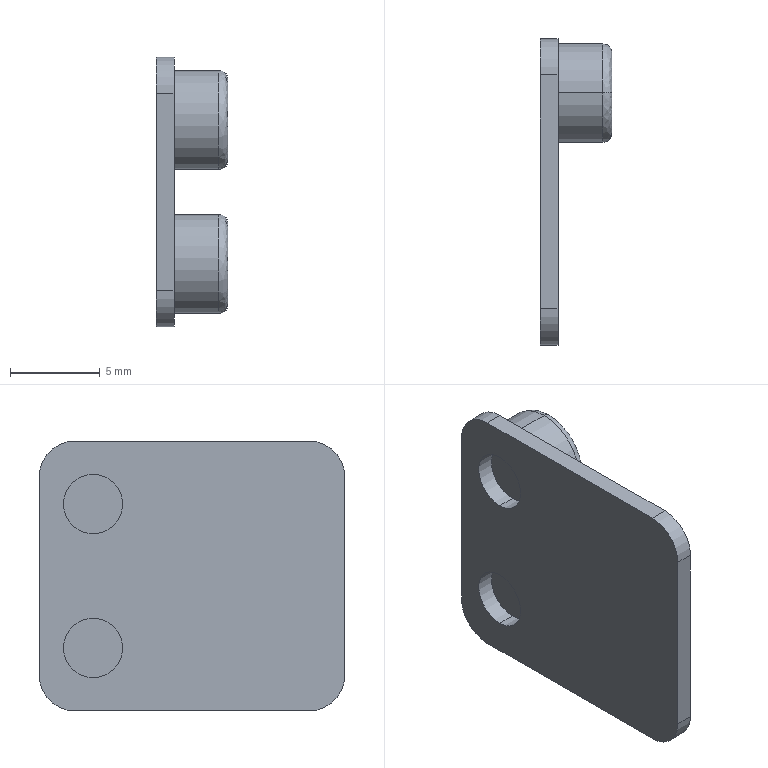Part | SolidWorks | features BaseBody 1 | 1 solid | 40 faces | box 4 x 17 x 15 mm | volume 361.162 mm3 | plane 24 | cylinder 12 | spline 4 | commonest cylinder face diameters 3.3 x4 4 x4 5.5 x4
STEP:
#1=CARTESIAN_POINT('',(4.,5.,1.25));
#2=VERTEX_POINT('',#1);
#3=CARTESIAN_POINT('',(4.,5.,5.75));
#4=VERTEX_POINT('',#3);
#5=CARTESIAN_POINT('',(4.,5.,1.25));
#6=CARTESIAN_POINT('',(4.,0.5,1.25));
#7=CARTESIAN_POINT('',(4.,0.5,5.75));
#8=CARTESIAN_POINT('',(4.,5.,5.75));
#9=(BOUNDED_CURVE()B_SPLINE_CURVE(3,(#5,#6,#7,#8),.UNSPECIFIED.,.F.,.T.)B_SPLINE_CURVE_WITH_KNOTS((4,4),(0.,0.5),.UNSPECIFIED.)CURVE()GEOMETRIC_REPRESENTATION_ITEM()RATIONAL_B_SPLINE_CURVE((1.,0.3333,0.3333,1.))REPRESENTATION_ITEM(''));
#10=EDGE_CURVE('',#2,#4,#9,.T.);
#11=ORIENTED_EDGE('',*,*,#10,.T.);
#12=CARTESIAN_POINT('',(3.5,5.,6.25));
#13=VERTEX_POINT('',#12);
#14=CARTESIAN_POINT('',(3.5,5.,5.75));
#15=DIRECTION('',(0.,-1.,0.));
#16=DIRECTION('',(0.,0.,1.));
#17=AXIS2_PLACEMENT_3D('',#14,#15,#16);
#18=CIRCLE('',#17,0.5);
#19=EDGE_CURVE('',#4,#13,#18,.T.);
#20=ORIENTED_EDGE('',*,*,#19,.T.);
#21=CARTESIAN_POINT('',(3.5,5.,0.75));
#22=VERTEX_POINT('',#21);
#23=CARTESIAN_POINT('',(3.5,5.,3.5));
#24=DIRECTION('',(-1.,0.,0.));
#25=DIRECTION('',(0.,0.,1.));
#26=AXIS2_PLACEMENT_3D('',#23,#24,#25);
#27=CIRCLE('',#26,2.75);
#28=EDGE_CURVE('',#22,#13,#27,.T.);
#29=ORIENTED_EDGE('',*,*,#28,.F.);
#30=CARTESIAN_POINT('',(3.5,5.,1.25));
#31=DIRECTION('',(0.,1.,0.));
#32=DIRECTION('',(0.,0.,-1.));
#33=AXIS2_PLACEMENT_3D('',#30,#31,#32);
#34=CIRCLE('',#33,0.5);
#35=EDGE_CURVE('',#2,#22,#34,.T.);
#36=ORIENTED_EDGE('',*,*,#35,.F.);
#37=EDGE_LOOP('',(#11,#20,#29,#36));
#38=FACE_OUTER_BOUND('',#37,.T.);
#39=CARTESIAN_POINT('',(4.,5.,5.75));
#40=CARTESIAN_POINT('',(4.,0.5,5.75));
#41=CARTESIAN_POINT('',(4.,0.5,1.25));
#42=CARTESIAN_POINT('',(4.,5.,1.25));
#43=CARTESIAN_POINT('',(4.,5.,6.043));
#44=CARTESIAN_POINT('',(4.,-0.08579,6.043));
#45=CARTESIAN_POINT('',(4.,-0.08579,0.9571));
#46=CARTESIAN_POINT('',(4.,5.,0.9571));
#47=CARTESIAN_POINT('',(3.793,5.,6.25));
#48=CARTESIAN_POINT('',(3.793,-0.5,6.25));
#49=CARTESIAN_POINT('',(3.793,-0.5,0.75));
#50=CARTESIAN_POINT('',(3.793,5.,0.75));
#51=CARTESIAN_POINT('',(3.5,5.,6.25));
#52=CARTESIAN_POINT('',(3.5,-0.5,6.25));
#53=CARTESIAN_POINT('',(3.5,-0.5,0.75));
#54=CARTESIAN_POINT('',(3.5,5.,0.75));
#55=(BOUNDED_SURFACE()B_SPLINE_SURFACE(3,3,((#39,#40,#41,#42),(#43,#44,#45,#46),(#47,#48,#49,#50),(#51,#52,#53,#54)),.UNSPECIFIED.,.F.,.F.,.F.)B_SPLINE_SURFACE_WITH_KNOTS((4,4),(4,4),(0.,1.),(0.,1.),.UNSPECIFIED.)GEOMETRIC_REPRESENTATION_ITEM()RATIONAL_B_SPLINE_SURFACE(((1.,0.3333,0.3333,1.),(0.8047,0.2682,0.2682,0.8047),(0.8047,0.2682,0.2682,0.8047),(1.,0.3333,0.3333,1.)))REPRESENTATION_ITEM('')SURFACE());
#56=ADVANCED_FACE('',(#38),#55,.T.);
#57=CARTESIAN_POINT('',(4.,5.,9.25));
#58=VERTEX_POINT('',#57);
#59=CARTESIAN_POINT('',(4.,5.,13.75));
#60=VERTEX_POINT('',#59);
#61=CARTESIAN_POINT('',(4.,5.,9.25));
#62=CARTESIAN_POINT('',(4.,0.5,9.25));
#63=CARTESIAN_POINT('',(4.,0.5,13.75));
#64=CARTESIAN_POINT('',(4.,5.,13.75));
#65=(BOUNDED_CURVE()B_SPLINE_CURVE(3,(#61,#62,#63,#64),.UNSPECIFIED.,.F.,.F.)B_SPLINE_CURVE_WITH_KNOTS((4,4),(0.,0.5),.UNSPECIFIED.)CURVE()GEOMETRIC_REPRESENTATION_ITEM()RATIONAL_B_SPLINE_CURVE((1.,0.3333,0.3333,1.))REPRESENTATION_ITEM(''));
#66=EDGE_CURVE('',#58,#60,#65,.T.);
#67=ORIENTED_EDGE('',*,*,#66,.T.);
#68=CARTESIAN_POINT('',(3.5,5.,14.25));
#69=VERTEX_POINT('',#68);
#70=CARTESIAN_POINT('',(3.5,5.,13.75));
#71=DIRECTION('',(0.,-1.,0.));
#72=DIRECTION('',(0.,0.,1.));
#73=AXIS2_PLACEMENT_3D('',#70,#71,#72);
#74=CIRCLE('',#73,0.5);
#75=EDGE_CURVE('',#60,#69,#74,.T.);
#76=ORIENTED_EDGE('',*,*,#75,.T.);
#77=CARTESIAN_POINT('',(3.5,5.,8.75));
#78=VERTEX_POINT('',#77);
#79=CARTESIAN_POINT('',(3.5,5.,11.5));
#80=DIRECTION('',(-1.,0.,0.));
#81=DIRECTION('',(0.,0.,1.));
#82=AXIS2_PLACEMENT_3D('',#79,#80,#81);
#83=CIRCLE('',#82,2.75);
#84=EDGE_CURVE('',#78,#69,#83,.T.);
#85=ORIENTED_EDGE('',*,*,#84,.F.);
#86=CARTESIAN_POINT('',(3.5,5.,9.25));
#87=DIRECTION('',(0.,1.,0.));
#88=DIRECTION('',(0.,0.,-1.));
#89=AXIS2_PLACEMENT_3D('',#86,#87,#88);
#90=CIRCLE('',#89,0.5);
#91=EDGE_CURVE('',#58,#78,#90,.T.);
#92=ORIENTED_EDGE('',*,*,#91,.F.);
#93=EDGE_LOOP('',(#67,#76,#85,#92));
#94=FACE_OUTER_BOUND('',#93,.T.);
#95=CARTESIAN_POINT('',(4.,5.,13.75));
#96=CARTESIAN_POINT('',(4.,0.5,13.75));
#97=CARTESIAN_POINT('',(4.,0.5,9.25));
#98=CARTESIAN_POINT('',(4.,5.,9.25));
#99=CARTESIAN_POINT('',(4.,5.,14.043));
#100=CARTESIAN_POINT('',(4.,-0.08579,14.043));
#101=CARTESIAN_POINT('',(4.,-0.08579,8.957));
#102=CARTESIAN_POINT('',(4.,5.,8.957));
#103=CARTESIAN_POINT('',(3.793,5.,14.25));
#104=CARTESIAN_POINT('',(3.793,-0.5,14.25));
#105=CARTESIAN_POINT('',(3.793,-0.5,8.75));
#106=CARTESIAN_POINT('',(3.793,5.,8.75));
#107=CARTESIAN_POINT('',(3.5,5.,14.25));
#108=CARTESIAN_POINT('',(3.5,-0.5,14.25));
#109=CARTESIAN_POINT('',(3.5,-0.5,8.75));
#110=CARTESIAN_POINT('',(3.5,5.,8.75));
#111=(BOUNDED_SURFACE()B_SPLINE_SURFACE(3,3,((#95,#96,#97,#98),(#99,#100,#101,#102),(#103,#104,#105,#106),(#107,#108,#109,#110)),.UNSPECIFIED.,.F.,.F.,.T.)B_SPLINE_SURFACE_WITH_KNOTS((4,4),(4,4),(0.,1.),(0.,1.),.UNSPECIFIED.)GEOMETRIC_REPRESENTATION_ITEM()RATIONAL_B_SPLINE_SURFACE(((1.,0.3333,0.3333,1.),(0.8047,0.2682,0.2682,0.8047),(0.8047,0.2682,0.2682,0.8047),(1.,0.3333,0.3333,1.)))REPRESENTATION_ITEM('')SURFACE());
#112=ADVANCED_FACE('',(#94),#111,.T.);
#113=CARTESIAN_POINT('',(0.,5.,1.85));
#114=VERTEX_POINT('',#113);
#115=CARTESIAN_POINT('',(0.,5.,5.15));
#116=VERTEX_POINT('',#115);
#117=CARTESIAN_POINT('',(0.,5.,3.5));
#118=DIRECTION('',(-1.,0.,0.));
#119=DIRECTION('',(0.,0.,-1.));
#120=AXIS2_PLACEMENT_3D('',#117,#118,#119);
#121=CIRCLE('',#120,1.65);
#122=EDGE_CURVE('',#114,#116,#121,.T.);
#123=ORIENTED_EDGE('',*,*,#122,.T.);
#124=CARTESIAN_POINT('',(1.,5.,5.15));
#125=VERTEX_POINT('',#124);
#126=CARTESIAN_POINT('',(0.,5.,5.15));
#127=DIRECTION('',(1.,0.,0.));
#128=VECTOR('',#127,1000.);
#129=LINE('',#126,#128);
#130=EDGE_CURVE('',#116,#125,#129,.T.);
#131=ORIENTED_EDGE('',*,*,#130,.T.);
#132=CARTESIAN_POINT('',(1.,5.,1.85));
#133=VERTEX_POINT('',#132);
#134=CARTESIAN_POINT('',(1.,5.,3.5));
#135=DIRECTION('',(-1.,0.,0.));
#136=DIRECTION('',(0.,0.,-1.));
#137=AXIS2_PLACEMENT_3D('',#134,#135,#136);
#138=CIRCLE('',#137,1.65);
#139=EDGE_CURVE('',#133,#125,#138,.T.);
#140=ORIENTED_EDGE('',*,*,#139,.F.);
#141=CARTESIAN_POINT('',(0.,5.,1.85));
#142=DIRECTION('',(1.,0.,0.));
#143=VECTOR('',#142,1000.);
#144=LINE('',#141,#143);
#145=EDGE_CURVE('',#114,#133,#144,.T.);
#146=ORIENTED_EDGE('',*,*,#145,.F.);
#147=EDGE_LOOP('',(#123,#131,#140,#146));
#148=FACE_OUTER_BOUND('',#147,.T.);
#149=CARTESIAN_POINT('',(0.,5.,3.5));
#150=DIRECTION('',(1.,0.,0.));
#151=DIRECTION('',(0.,0.,-1.));
#152=AXIS2_PLACEMENT_3D('',#149,#150,#151);
#153=CYLINDRICAL_SURFACE('',#152,1.65);
#154=ADVANCED_FACE('',(#148),#153,.F.);
#155=CARTESIAN_POINT('',(0.,5.,9.85));
#156=VERTEX_POINT('',#155);
#157=CARTESIAN_POINT('',(0.,5.,13.15));
#158=VERTEX_POINT('',#157);
#159=CARTESIAN_POINT('',(0.,5.,11.5));
#160=DIRECTION('',(-1.,0.,0.));
#161=DIRECTION('',(0.,0.,-1.));
#162=AXIS2_PLACEMENT_3D('',#159,#160,#161);
#163=CIRCLE('',#162,1.65);
#164=EDGE_CURVE('',#156,#158,#163,.T.);
#165=ORIENTED_EDGE('',*,*,#164,.T.);
#166=CARTESIAN_POINT('',(1.,5.,13.15));
#167=VERTEX_POINT('',#166);
#168=CARTESIAN_POINT('',(0.,5.,13.15));
#169=DIRECTION('',(1.,0.,0.));
#170=VECTOR('',#169,1000.);
#171=LINE('',#168,#170);
#172=EDGE_CURVE('',#158,#167,#171,.T.);
#173=ORIENTED_EDGE('',*,*,#172,.T.);
#174=CARTESIAN_POINT('',(1.,5.,9.85));
#175=VERTEX_POINT('',#174);
#176=CARTESIAN_POINT('',(1.,5.,11.5));
#177=DIRECTION('',(-1.,0.,0.));
#178=DIRECTION('',(0.,0.,-1.));
#179=AXIS2_PLACEMENT_3D('',#176,#177,#178);
#180=CIRCLE('',#179,1.65);
#181=EDGE_CURVE('',#175,#167,#180,.T.);
#182=ORIENTED_EDGE('',*,*,#181,.F.);
#183=CARTESIAN_POINT('',(0.,5.,9.85));
#184=DIRECTION('',(1.,0.,0.));
#185=VECTOR('',#184,1000.);
#186=LINE('',#183,#185);
#187=EDGE_CURVE('',#156,#175,#186,.T.);
#188=ORIENTED_EDGE('',*,*,#187,.F.);
#189=EDGE_LOOP('',(#165,#173,#182,#188));
#190=FACE_OUTER_BOUND('',#189,.T.);
#191=CARTESIAN_POINT('',(0.,5.,11.5));
#192=DIRECTION('',(1.,0.,0.));
#193=DIRECTION('',(0.,0.,-1.));
#194=AXIS2_PLACEMENT_3D('',#191,#192,#193);
#195=CYLINDRICAL_SURFACE('',#194,1.65);
#196=ADVANCED_FACE('',(#190),#195,.F.);
#197=CARTESIAN_POINT('',(3.5,5.,3.5));
#198=DIRECTION('',(-1.,0.,0.));
#199=DIRECTION('',(0.,0.,1.));
#200=AXIS2_PLACEMENT_3D('',#197,#198,#199);
#201=CIRCLE('',#200,2.75);
#202=EDGE_CURVE('',#13,#22,#201,.T.);
#203=ORIENTED_EDGE('',*,*,#202,.T.);
#204=CARTESIAN_POINT('',(1.,5.,0.75));
#205=VERTEX_POINT('',#204);
#206=CARTESIAN_POINT('',(4.,5.,0.75));
#207=DIRECTION('',(-1.,0.,0.));
#208=VECTOR('',#207,1000.);
#209=LINE('',#206,#208);
#210=EDGE_CURVE('',#22,#205,#209,.T.);
#211=ORIENTED_EDGE('',*,*,#210,.T.);
#212=CARTESIAN_POINT('',(1.,5.,6.25));
#213=VERTEX_POINT('',#212);
#214=CARTESIAN_POINT('',(1.,5.,3.5));
#215=DIRECTION('',(-1.,0.,0.));
#216=DIRECTION('',(0.,0.,1.));
#217=AXIS2_PLACEMENT_3D('',#214,#215,#216);
#218=CIRCLE('',#217,2.75);
#219=EDGE_CURVE('',#213,#205,#218,.T.);
#220=ORIENTED_EDGE('',*,*,#219,.F.);
#221=CARTESIAN_POINT('',(4.,5.,6.25));
#222=DIRECTION('',(-1.,0.,0.));
#223=VECTOR('',#222,1000.);
#224=LINE('',#221,#223);
#225=EDGE_CURVE('',#13,#213,#224,.T.);
#226=ORIENTED_EDGE('',*,*,#225,.F.);
#227=EDGE_LOOP('',(#203,#211,#220,#226));
#228=FACE_OUTER_BOUND('',#227,.T.);
#229=CARTESIAN_POINT('',(4.,5.,3.5));
#230=DIRECTION('',(-1.,0.,0.));
#231=DIRECTION('',(0.,0.,1.));
#232=AXIS2_PLACEMENT_3D('',#229,#230,#231);
#233=CYLINDRICAL_SURFACE('',#232,2.75);
#234=ADVANCED_FACE('',(#228),#233,.T.);
#235=CARTESIAN_POINT('',(3.5,5.,11.5));
#236=DIRECTION('',(-1.,0.,0.));
#237=DIRECTION('',(0.,0.,1.));
#238=AXIS2_PLACEMENT_3D('',#235,#236,#237);
#239=CIRCLE('',#238,2.75);
#240=EDGE_CURVE('',#69,#78,#239,.T.);
#241=ORIENTED_EDGE('',*,*,#240,.T.);
#242=CARTESIAN_POINT('',(1.,5.,8.75));
#243=VERTEX_POINT('',#242);
#244=CARTESIAN_POINT('',(4.,5.,8.75));
#245=DIRECTION('',(-1.,0.,0.));
#246=VECTOR('',#245,1000.);
#247=LINE('',#244,#246);
#248=EDGE_CURVE('',#78,#243,#247,.T.);
#249=ORIENTED_EDGE('',*,*,#248,.T.);
#250=CARTESIAN_POINT('',(1.,5.,14.25));
#251=VERTEX_POINT('',#250);
#252=CARTESIAN_POINT('',(1.,5.,11.5));
#253=DIRECTION('',(-1.,0.,0.));
#254=DIRECTION('',(0.,0.,1.));
#255=AXIS2_PLACEMENT_3D('',#252,#253,#254);
#256=CIRCLE('',#255,2.75);
#257=EDGE_CURVE('',#251,#243,#256,.T.);
#258=ORIENTED_EDGE('',*,*,#257,.F.);
#259=CARTESIAN_POINT('',(4.,5.,14.25));
#260=DIRECTION('',(-1.,0.,0.));
#261=VECTOR('',#260,1000.);
#262=LINE('',#259,#261);
#263=EDGE_CURVE('',#69,#251,#262,.T.);
#264=ORIENTED_EDGE('',*,*,#263,.F.);
#265=EDGE_LOOP('',(#241,#249,#258,#264));
#266=FACE_OUTER_BOUND('',#265,.T.);
#267=CARTESIAN_POINT('',(4.,5.,11.5));
#268=DIRECTION('',(-1.,0.,0.));
#269=DIRECTION('',(0.,0.,1.));
#270=AXIS2_PLACEMENT_3D('',#267,#268,#269);
#271=CYLINDRICAL_SURFACE('',#270,2.75);
#272=ADVANCED_FACE('',(#266),#271,.T.);
#273=CARTESIAN_POINT('',(0.,-7.,15.));
#274=VERTEX_POINT('',#273);
#275=CARTESIAN_POINT('',(0.,-9.,13.));
#276=VERTEX_POINT('',#275);
#277=CARTESIAN_POINT('',(0.,-7.,13.));
#278=DIRECTION('',(1.,0.,0.));
#279=DIRECTION('',(0.,0.,1.));
#280=AXIS2_PLACEMENT_3D('',#277,#278,#279);
#281=CIRCLE('',#280,2.);
#282=EDGE_CURVE('',#274,#276,#281,.T.);
#283=ORIENTED_EDGE('',*,*,#282,.F.);
#284=CARTESIAN_POINT('',(0.,6.,15.));
#285=VERTEX_POINT('',#284);
#286=CARTESIAN_POINT('',(0.,-0.5,15.));
#287=DIRECTION('',(0.,-1.,0.));
#288=VECTOR('',#287,1000.);
#289=LINE('',#286,#288);
#290=EDGE_CURVE('',#285,#274,#289,.T.);
#291=ORIENTED_EDGE('',*,*,#290,.F.);
#292=CARTESIAN_POINT('',(0.,8.,13.));
#293=VERTEX_POINT('',#292);
#294=CARTESIAN_POINT('',(0.,6.,13.));
#295=DIRECTION('',(1.,0.,0.));
#296=DIRECTION('',(0.,0.,1.));
#297=AXIS2_PLACEMENT_3D('',#294,#295,#296);
#298=CIRCLE('',#297,2.);
#299=EDGE_CURVE('',#293,#285,#298,.T.);
#300=ORIENTED_EDGE('',*,*,#299,.F.);
#301=CARTESIAN_POINT('',(0.,8.,2.));
#302=VERTEX_POINT('',#301);
#303=CARTESIAN_POINT('',(0.,8.,7.5));
#304=DIRECTION('',(0.,0.,1.));
#305=VECTOR('',#304,1000.);
#306=LINE('',#303,#305);
#307=EDGE_CURVE('',#302,#293,#306,.T.);
#308=ORIENTED_EDGE('',*,*,#307,.F.);
#309=CARTESIAN_POINT('',(0.,6.,0.));
#310=VERTEX_POINT('',#309);
#311=CARTESIAN_POINT('',(0.,6.,2.));
#312=DIRECTION('',(1.,0.,0.));
#313=DIRECTION('',(0.,0.,1.));
#314=AXIS2_PLACEMENT_3D('',#311,#312,#313);
#315=CIRCLE('',#314,2.);
#316=EDGE_CURVE('',#310,#302,#315,.T.);
#317=ORIENTED_EDGE('',*,*,#316,.F.);
#318=CARTESIAN_POINT('',(0.,-7.,0.));
#319=VERTEX_POINT('',#318);
#320=CARTESIAN_POINT('',(0.,-0.5,0.));
#321=DIRECTION('',(0.,1.,0.));
#322=VECTOR('',#321,1000.);
#323=LINE('',#320,#322);
#324=EDGE_CURVE('',#319,#310,#323,.T.);
#325=ORIENTED_EDGE('',*,*,#324,.F.);
#326=CARTESIAN_POINT('',(0.,-9.,2.));
#327=VERTEX_POINT('',#326);
#328=CARTESIAN_POINT('',(0.,-7.,2.));
#329=DIRECTION('',(1.,0.,0.));
#330=DIRECTION('',(0.,0.,1.));
#331=AXIS2_PLACEMENT_3D('',#328,#329,#330);
#332=CIRCLE('',#331,2.);
#333=EDGE_CURVE('',#327,#319,#332,.T.);
#334=ORIENTED_EDGE('',*,*,#333,.F.);
#335=CARTESIAN_POINT('',(0.,-9.,7.5));
#336=DIRECTION('',(0.,0.,-1.));
#337=VECTOR('',#336,1000.);
#338=LINE('',#335,#337);
#339=EDGE_CURVE('',#276,#327,#338,.T.);
#340=ORIENTED_EDGE('',*,*,#339,.F.);
#341=EDGE_LOOP('',(#283,#291,#300,#308,#317,#325,#334,#340));
#342=FACE_OUTER_BOUND('',#341,.T.);
#343=ORIENTED_EDGE('',*,*,#122,.F.);
#344=CARTESIAN_POINT('',(0.,5.,3.5));
#345=DIRECTION('',(-1.,0.,0.));
#346=DIRECTION('',(0.,0.,-1.));
#347=AXIS2_PLACEMENT_3D('',#344,#345,#346);
#348=CIRCLE('',#347,1.65);
#349=EDGE_CURVE('',#116,#114,#348,.T.);
#350=ORIENTED_EDGE('',*,*,#349,.F.);
#351=EDGE_LOOP('',(#343,#350));
#352=FACE_BOUND('',#351,.T.);
#353=ORIENTED_EDGE('',*,*,#164,.F.);
#354=CARTESIAN_POINT('',(0.,5.,11.5));
#355=DIRECTION('',(-1.,0.,0.));
#356=DIRECTION('',(0.,0.,-1.));
#357=AXIS2_PLACEMENT_3D('',#354,#355,#356);
#358=CIRCLE('',#357,1.65);
#359=EDGE_CURVE('',#158,#156,#358,.T.);
#360=ORIENTED_EDGE('',*,*,#359,.F.);
#361=EDGE_LOOP('',(#353,#360));
#362=FACE_BOUND('',#361,.T.);
#363=CARTESIAN_POINT('',(0.,-0.5,7.5));
#364=DIRECTION('',(1.,0.,0.));
#365=DIRECTION('',(0.,0.,-1.));
#366=AXIS2_PLACEMENT_3D('',#363,#364,#365);
#367=PLANE('',#366);
#368=ADVANCED_FACE('',(#342,#352,#362),#367,.F.);
#369=CARTESIAN_POINT('',(1.,-9.,2.));
#370=VERTEX_POINT('',#369);
#371=CARTESIAN_POINT('',(1.,-9.,2.));
#372=DIRECTION('',(1.,0.,0.));
#373=VECTOR('',#372,1000.);
#374=LINE('',#371,#373);
#375=EDGE_CURVE('',#327,#370,#374,.T.);
#376=ORIENTED_EDGE('',*,*,#375,.T.);
#377=CARTESIAN_POINT('',(1.,-9.,13.));
#378=VERTEX_POINT('',#377);
#379=CARTESIAN_POINT('',(1.,-9.,15.));
#380=DIRECTION('',(0.,0.,1.));
#381=VECTOR('',#380,1000.);
#382=LINE('',#379,#381);
#383=EDGE_CURVE('',#370,#378,#382,.T.);
#384=ORIENTED_EDGE('',*,*,#383,.T.);
#385=CARTESIAN_POINT('',(1.,-9.,13.));
#386=DIRECTION('',(-1.,0.,0.));
#387=VECTOR('',#386,1000.);
#388=LINE('',#385,#387);
#389=EDGE_CURVE('',#378,#276,#388,.T.);
#390=ORIENTED_EDGE('',*,*,#389,.T.);
#391=ORIENTED_EDGE('',*,*,#339,.T.);
#392=EDGE_LOOP('',(#376,#384,#390,#391));
#393=FACE_OUTER_BOUND('',#392,.T.);
#394=CARTESIAN_POINT('',(1.,-9.,15.));
#395=DIRECTION('',(0.,-1.,0.));
#396=DIRECTION('',(0.,0.,-1.));
#397=AXIS2_PLACEMENT_3D('',#394,#395,#396);
#398=PLANE('',#397);
#399=ADVANCED_FACE('',(#393),#398,.T.);
#400=ORIENTED_EDGE('',*,*,#282,.T.);
#401=ORIENTED_EDGE('',*,*,#389,.F.);
#402=CARTESIAN_POINT('',(1.,-7.,15.));
#403=VERTEX_POINT('',#402);
#404=CARTESIAN_POINT('',(1.,-7.,13.));
#405=DIRECTION('',(-1.,0.,0.));
#406=DIRECTION('',(0.,0.,1.));
#407=AXIS2_PLACEMENT_3D('',#404,#405,#406);
#408=CIRCLE('',#407,2.);
#409=EDGE_CURVE('',#378,#403,#408,.T.);
#410=ORIENTED_EDGE('',*,*,#409,.T.);
#411=CARTESIAN_POINT('',(1.,-7.,15.));
#412=DIRECTION('',(-1.,0.,0.));
#413=VECTOR('',#412,1000.);
#414=LINE('',#411,#413);
#415=EDGE_CURVE('',#403,#274,#414,.T.);
#416=ORIENTED_EDGE('',*,*,#415,.T.);
#417=EDGE_LOOP('',(#400,#401,#410,#416));
#418=FACE_OUTER_BOUND('',#417,.T.);
#419=CARTESIAN_POINT('',(1.,-7.,13.));
#420=DIRECTION('',(-1.,0.,0.));
#421=DIRECTION('',(0.,0.,1.));
#422=AXIS2_PLACEMENT_3D('',#419,#420,#421);
#423=CYLINDRICAL_SURFACE('',#422,2.);
#424=ADVANCED_FACE('',(#418),#423,.T.);
#425=ORIENTED_EDGE('',*,*,#415,.F.);
#426=CARTESIAN_POINT('',(1.,6.,15.));
#427=VERTEX_POINT('',#426);
#428=CARTESIAN_POINT('',(1.,8.,15.));
#429=DIRECTION('',(0.,1.,0.));
#430=VECTOR('',#429,1000.);
#431=LINE('',#428,#430);
#432=EDGE_CURVE('',#403,#427,#431,.T.);
#433=ORIENTED_EDGE('',*,*,#432,.T.);
#434=CARTESIAN_POINT('',(1.,6.,15.));
#435=DIRECTION('',(-1.,0.,0.));
#436=VECTOR('',#435,1000.);
#437=LINE('',#434,#436);
#438=EDGE_CURVE('',#427,#285,#437,.T.);
#439=ORIENTED_EDGE('',*,*,#438,.T.);
#440=ORIENTED_EDGE('',*,*,#290,.T.);
#441=EDGE_LOOP('',(#425,#433,#439,#440));
#442=FACE_OUTER_BOUND('',#441,.T.);
#443=CARTESIAN_POINT('',(1.,8.,15.));
#444=DIRECTION('',(0.,0.,1.));
#445=DIRECTION('',(1.,0.,0.));
#446=AXIS2_PLACEMENT_3D('',#443,#444,#445);
#447=PLANE('',#446);
#448=ADVANCED_FACE('',(#442),#447,.T.);
#449=ORIENTED_EDGE('',*,*,#299,.T.);
#450=ORIENTED_EDGE('',*,*,#438,.F.);
#451=CARTESIAN_POINT('',(1.,8.,13.));
#452=VERTEX_POINT('',#451);
#453=CARTESIAN_POINT('',(1.,6.,13.));
#454=DIRECTION('',(-1.,0.,0.));
#455=DIRECTION('',(0.,0.,1.));
#456=AXIS2_PLACEMENT_3D('',#453,#454,#455);
#457=CIRCLE('',#456,2.);
#458=EDGE_CURVE('',#427,#452,#457,.T.);
#459=ORIENTED_EDGE('',*,*,#458,.T.);
#460=CARTESIAN_POINT('',(1.,8.,13.));
#461=DIRECTION('',(-1.,0.,0.));
#462=VECTOR('',#461,1000.);
#463=LINE('',#460,#462);
#464=EDGE_CURVE('',#452,#293,#463,.T.);
#465=ORIENTED_EDGE('',*,*,#464,.T.);
#466=EDGE_LOOP('',(#449,#450,#459,#465));
#467=FACE_OUTER_BOUND('',#466,.T.);
#468=CARTESIAN_POINT('',(1.,6.,13.));
#469=DIRECTION('',(-1.,0.,0.));
#470=DIRECTION('',(0.,0.,1.));
#471=AXIS2_PLACEMENT_3D('',#468,#469,#470);
#472=CYLINDRICAL_SURFACE('',#471,2.);
#473=ADVANCED_FACE('',(#467),#472,.T.);
#474=CARTESIAN_POINT('',(1.,8.,2.));
#475=VERTEX_POINT('',#474);
#476=CARTESIAN_POINT('',(1.,8.,2.));
#477=DIRECTION('',(-1.,0.,0.));
#478=VECTOR('',#477,1000.);
#479=LINE('',#476,#478);
#480=EDGE_CURVE('',#475,#302,#479,.T.);
#481=ORIENTED_EDGE('',*,*,#480,.T.);
#482=ORIENTED_EDGE('',*,*,#307,.T.);
#483=ORIENTED_EDGE('',*,*,#464,.F.);
#484=CARTESIAN_POINT('',(1.,8.,0.));
#485=DIRECTION('',(0.,0.,-1.));
#486=VECTOR('',#485,1000.);
#487=LINE('',#484,#486);
#488=EDGE_CURVE('',#452,#475,#487,.T.);
#489=ORIENTED_EDGE('',*,*,#488,.T.);
#490=EDGE_LOOP('',(#481,#482,#483,#489));
#491=FACE_OUTER_BOUND('',#490,.T.);
#492=CARTESIAN_POINT('',(1.,8.,0.));
#493=DIRECTION('',(0.,1.,0.));
#494=DIRECTION('',(0.,0.,1.));
#495=AXIS2_PLACEMENT_3D('',#492,#493,#494);
#496=PLANE('',#495);
#497=ADVANCED_FACE('',(#491),#496,.T.);
#498=ORIENTED_EDGE('',*,*,#316,.T.);
#499=ORIENTED_EDGE('',*,*,#480,.F.);
#500=CARTESIAN_POINT('',(1.,6.,0.));
#501=VERTEX_POINT('',#500);
#502=CARTESIAN_POINT('',(1.,6.,2.));
#503=DIRECTION('',(-1.,0.,0.));
#504=DIRECTION('',(0.,0.,1.));
#505=AXIS2_PLACEMENT_3D('',#502,#503,#504);
#506=CIRCLE('',#505,2.);
#507=EDGE_CURVE('',#475,#501,#506,.T.);
#508=ORIENTED_EDGE('',*,*,#507,.T.);
#509=CARTESIAN_POINT('',(1.,6.,0.));
#510=DIRECTION('',(-1.,0.,0.));
#511=VECTOR('',#510,1000.);
#512=LINE('',#509,#511);
#513=EDGE_CURVE('',#501,#310,#512,.T.);
#514=ORIENTED_EDGE('',*,*,#513,.T.);
#515=EDGE_LOOP('',(#498,#499,#508,#514));
#516=FACE_OUTER_BOUND('',#515,.T.);
#517=CARTESIAN_POINT('',(1.,6.,2.));
#518=DIRECTION('',(-1.,0.,0.));
#519=DIRECTION('',(0.,0.,1.));
#520=AXIS2_PLACEMENT_3D('',#517,#518,#519);
#521=CYLINDRICAL_SURFACE('',#520,2.);
#522=ADVANCED_FACE('',(#516),#521,.T.);
#523=CARTESIAN_POINT('',(1.,-7.,0.));
#524=VERTEX_POINT('',#523);
#525=CARTESIAN_POINT('',(1.,-7.,0.));
#526=DIRECTION('',(-1.,0.,0.));
#527=VECTOR('',#526,1000.);
#528=LINE('',#525,#527);
#529=EDGE_CURVE('',#524,#319,#528,.T.);
#530=ORIENTED_EDGE('',*,*,#529,.T.);
#531=ORIENTED_EDGE('',*,*,#324,.T.);
#532=ORIENTED_EDGE('',*,*,#513,.F.);
#533=CARTESIAN_POINT('',(1.,-9.,0.));
#534=DIRECTION('',(0.,-1.,0.));
#535=VECTOR('',#534,1000.);
#536=LINE('',#533,#535);
#537=EDGE_CURVE('',#501,#524,#536,.T.);
#538=ORIENTED_EDGE('',*,*,#537,.T.);
#539=EDGE_LOOP('',(#530,#531,#532,#538));
#540=FACE_OUTER_BOUND('',#539,.T.);
#541=CARTESIAN_POINT('',(1.,-9.,0.));
#542=DIRECTION('',(0.,0.,-1.));
#543=DIRECTION('',(-1.,0.,0.));
#544=AXIS2_PLACEMENT_3D('',#541,#542,#543);
#545=PLANE('',#544);
#546=ADVANCED_FACE('',(#540),#545,.T.);
#547=ORIENTED_EDGE('',*,*,#333,.T.);
#548=ORIENTED_EDGE('',*,*,#529,.F.);
#549=CARTESIAN_POINT('',(1.,-7.,2.));
#550=DIRECTION('',(-1.,0.,0.));
#551=DIRECTION('',(0.,0.,1.));
#552=AXIS2_PLACEMENT_3D('',#549,#550,#551);
#553=CIRCLE('',#552,2.);
#554=EDGE_CURVE('',#524,#370,#553,.T.);
#555=ORIENTED_EDGE('',*,*,#554,.T.);
#556=ORIENTED_EDGE('',*,*,#375,.F.);
#557=EDGE_LOOP('',(#547,#548,#555,#556));
#558=FACE_OUTER_BOUND('',#557,.T.);
#559=CARTESIAN_POINT('',(1.,-7.,2.));
#560=DIRECTION('',(-1.,0.,0.));
#561=DIRECTION('',(0.,0.,1.));
#562=AXIS2_PLACEMENT_3D('',#559,#560,#561);
#563=CYLINDRICAL_SURFACE('',#562,2.);
#564=ADVANCED_FACE('',(#558),#563,.T.);
#565=ORIENTED_EDGE('',*,*,#130,.F.);
#566=ORIENTED_EDGE('',*,*,#349,.T.);
#567=ORIENTED_EDGE('',*,*,#145,.T.);
#568=CARTESIAN_POINT('',(1.,5.,3.5));
#569=DIRECTION('',(-1.,0.,0.));
#570=DIRECTION('',(0.,0.,-1.));
#571=AXIS2_PLACEMENT_3D('',#568,#569,#570);
#572=CIRCLE('',#571,1.65);
#573=EDGE_CURVE('',#125,#133,#572,.T.);
#574=ORIENTED_EDGE('',*,*,#573,.F.);
#575=EDGE_LOOP('',(#565,#566,#567,#574));
#576=FACE_OUTER_BOUND('',#575,.T.);
#577=CARTESIAN_POINT('',(0.,5.,3.5));
#578=DIRECTION('',(1.,0.,0.));
#579=DIRECTION('',(0.,0.,-1.));
#580=AXIS2_PLACEMENT_3D('',#577,#578,#579);
#581=CYLINDRICAL_SURFACE('',#580,1.65);
#582=ADVANCED_FACE('',(#576),#581,.F.);
#583=ORIENTED_EDGE('',*,*,#172,.F.);
#584=ORIENTED_EDGE('',*,*,#359,.T.);
#585=ORIENTED_EDGE('',*,*,#187,.T.);
#586=CARTESIAN_POINT('',(1.,5.,11.5));
#587=DIRECTION('',(-1.,0.,0.));
#588=DIRECTION('',(0.,0.,-1.));
#589=AXIS2_PLACEMENT_3D('',#586,#587,#588);
#590=CIRCLE('',#589,1.65);
#591=EDGE_CURVE('',#167,#175,#590,.T.);
#592=ORIENTED_EDGE('',*,*,#591,.F.);
#593=EDGE_LOOP('',(#583,#584,#585,#592));
#594=FACE_OUTER_BOUND('',#593,.T.);
#595=CARTESIAN_POINT('',(0.,5.,11.5));
#596=DIRECTION('',(1.,0.,0.));
#597=DIRECTION('',(0.,0.,-1.));
#598=AXIS2_PLACEMENT_3D('',#595,#596,#597);
#599=CYLINDRICAL_SURFACE('',#598,1.65);
#600=ADVANCED_FACE('',(#594),#599,.F.);
#601=ORIENTED_EDGE('',*,*,#219,.T.);
#602=CARTESIAN_POINT('',(1.,5.,3.5));
#603=DIRECTION('',(-1.,0.,0.));
#604=DIRECTION('',(0.,0.,1.));
#605=AXIS2_PLACEMENT_3D('',#602,#603,#604);
#606=CIRCLE('',#605,2.75);
#607=EDGE_CURVE('',#205,#213,#606,.T.);
#608=ORIENTED_EDGE('',*,*,#607,.T.);
#609=EDGE_LOOP('',(#601,#608));
#610=FACE_BOUND('',#609,.T.);
#611=ORIENTED_EDGE('',*,*,#458,.F.);
#612=ORIENTED_EDGE('',*,*,#432,.F.);
#613=ORIENTED_EDGE('',*,*,#409,.F.);
#614=ORIENTED_EDGE('',*,*,#383,.F.);
#615=ORIENTED_EDGE('',*,*,#554,.F.);
#616=ORIENTED_EDGE('',*,*,#537,.F.);
#617=ORIENTED_EDGE('',*,*,#507,.F.);
#618=ORIENTED_EDGE('',*,*,#488,.F.);
#619=EDGE_LOOP('',(#611,#612,#613,#614,#615,#616,#617,#618));
#620=FACE_OUTER_BOUND('',#619,.T.);
#621=ORIENTED_EDGE('',*,*,#257,.T.);
#622=CARTESIAN_POINT('',(1.,5.,11.5));
#623=DIRECTION('',(-1.,0.,0.));
#624=DIRECTION('',(0.,0.,1.));
#625=AXIS2_PLACEMENT_3D('',#622,#623,#624);
#626=CIRCLE('',#625,2.75);
#627=EDGE_CURVE('',#243,#251,#626,.T.);
#628=ORIENTED_EDGE('',*,*,#627,.T.);
#629=EDGE_LOOP('',(#621,#628));
#630=FACE_BOUND('',#629,.T.);
#631=CARTESIAN_POINT('',(1.,-0.5,7.5));
#632=DIRECTION('',(1.,0.,0.));
#633=DIRECTION('',(0.,0.,-1.));
#634=AXIS2_PLACEMENT_3D('',#631,#632,#633);
#635=PLANE('',#634);
#636=ADVANCED_FACE('',(#610,#620,#630),#635,.T.);
#637=ORIENTED_EDGE('',*,*,#139,.T.);
#638=ORIENTED_EDGE('',*,*,#573,.T.);
#639=EDGE_LOOP('',(#637,#638));
#640=FACE_OUTER_BOUND('',#639,.T.);
#641=CARTESIAN_POINT('',(1.,5.,3.5));
#642=DIRECTION('',(1.,0.,0.));
#643=DIRECTION('',(0.,0.,-1.));
#644=AXIS2_PLACEMENT_3D('',#641,#642,#643);
#645=PLANE('',#644);
#646=ADVANCED_FACE('',(#640),#645,.F.);
#647=ORIENTED_EDGE('',*,*,#181,.T.);
#648=ORIENTED_EDGE('',*,*,#591,.T.);
#649=EDGE_LOOP('',(#647,#648));
#650=FACE_OUTER_BOUND('',#649,.T.);
#651=CARTESIAN_POINT('',(1.,5.,11.5));
#652=DIRECTION('',(1.,0.,0.));
#653=DIRECTION('',(0.,0.,-1.));
#654=AXIS2_PLACEMENT_3D('',#651,#652,#653);
#655=PLANE('',#654);
#656=ADVANCED_FACE('',(#650),#655,.F.);
#657=ORIENTED_EDGE('',*,*,#210,.F.);
#658=ORIENTED_EDGE('',*,*,#28,.T.);
#659=ORIENTED_EDGE('',*,*,#225,.T.);
#660=ORIENTED_EDGE('',*,*,#607,.F.);
#661=EDGE_LOOP('',(#657,#658,#659,#660));
#662=FACE_OUTER_BOUND('',#661,.T.);
#663=CARTESIAN_POINT('',(4.,5.,3.5));
#664=DIRECTION('',(-1.,0.,0.));
#665=DIRECTION('',(0.,0.,1.));
#666=AXIS2_PLACEMENT_3D('',#663,#664,#665);
#667=CYLINDRICAL_SURFACE('',#666,2.75);
#668=ADVANCED_FACE('',(#662),#667,.T.);
#669=ORIENTED_EDGE('',*,*,#248,.F.);
#670=ORIENTED_EDGE('',*,*,#84,.T.);
#671=ORIENTED_EDGE('',*,*,#263,.T.);
#672=ORIENTED_EDGE('',*,*,#627,.F.);
#673=EDGE_LOOP('',(#669,#670,#671,#672));
#674=FACE_OUTER_BOUND('',#673,.T.);
#675=CARTESIAN_POINT('',(4.,5.,11.5));
#676=DIRECTION('',(-1.,0.,0.));
#677=DIRECTION('',(0.,0.,1.));
#678=AXIS2_PLACEMENT_3D('',#675,#676,#677);
#679=CYLINDRICAL_SURFACE('',#678,2.75);
#680=ADVANCED_FACE('',(#674),#679,.T.);
#681=ORIENTED_EDGE('',*,*,#19,.F.);
#682=CARTESIAN_POINT('',(4.,5.,5.75));
#683=CARTESIAN_POINT('',(4.,9.5,5.75));
#684=CARTESIAN_POINT('',(4.,9.5,1.25));
#685=CARTESIAN_POINT('',(4.,5.,1.25));
#686=(BOUNDED_CURVE()B_SPLINE_CURVE(3,(#682,#683,#684,#685),.UNSPECIFIED.,.F.,.F.)B_SPLINE_CURVE_WITH_KNOTS((4,4),(0.5,1.),.UNSPECIFIED.)CURVE()GEOMETRIC_REPRESENTATION_ITEM()RATIONAL_B_SPLINE_CURVE((1.,0.3333,0.3333,1.))REPRESENTATION_ITEM(''));
#687=EDGE_CURVE('',#4,#2,#686,.T.);
#688=ORIENTED_EDGE('',*,*,#687,.T.);
#689=ORIENTED_EDGE('',*,*,#35,.T.);
#690=ORIENTED_EDGE('',*,*,#202,.F.);
#691=EDGE_LOOP('',(#681,#688,#689,#690));
#692=FACE_OUTER_BOUND('',#691,.T.);
#693=CARTESIAN_POINT('',(4.,5.,1.25));
#694=CARTESIAN_POINT('',(4.,9.5,1.25));
#695=CARTESIAN_POINT('',(4.,9.5,5.75));
#696=CARTESIAN_POINT('',(4.,5.,5.75));
#697=CARTESIAN_POINT('',(4.,5.,0.9571));
#698=CARTESIAN_POINT('',(4.,10.086,0.9571));
#699=CARTESIAN_POINT('',(4.,10.086,6.043));
#700=CARTESIAN_POINT('',(4.,5.,6.043));
#701=CARTESIAN_POINT('',(3.793,5.,0.75));
#702=CARTESIAN_POINT('',(3.793,10.5,0.75));
#703=CARTESIAN_POINT('',(3.793,10.5,6.25));
#704=CARTESIAN_POINT('',(3.793,5.,6.25));
#705=CARTESIAN_POINT('',(3.5,5.,0.75));
#706=CARTESIAN_POINT('',(3.5,10.5,0.75));
#707=CARTESIAN_POINT('',(3.5,10.5,6.25));
#708=CARTESIAN_POINT('',(3.5,5.,6.25));
#709=(BOUNDED_SURFACE()B_SPLINE_SURFACE(3,3,((#693,#694,#695,#696),(#697,#698,#699,#700),(#701,#702,#703,#704),(#705,#706,#707,#708)),.UNSPECIFIED.,.F.,.F.,.F.)B_SPLINE_SURFACE_WITH_KNOTS((4,4),(4,4),(0.,1.),(0.,1.),.UNSPECIFIED.)GEOMETRIC_REPRESENTATION_ITEM()RATIONAL_B_SPLINE_SURFACE(((1.,0.3333,0.3333,1.),(0.8047,0.2682,0.2682,0.8047),(0.8047,0.2682,0.2682,0.8047),(1.,0.3333,0.3333,1.)))REPRESENTATION_ITEM('')SURFACE());
#710=ADVANCED_FACE('',(#692),#709,.T.);
#711=ORIENTED_EDGE('',*,*,#75,.F.);
#712=CARTESIAN_POINT('',(4.,5.,13.75));
#713=CARTESIAN_POINT('',(4.,9.5,13.75));
#714=CARTESIAN_POINT('',(4.,9.5,9.25));
#715=CARTESIAN_POINT('',(4.,5.,9.25));
#716=(BOUNDED_CURVE()B_SPLINE_CURVE(3,(#712,#713,#714,#715),.UNSPECIFIED.,.F.,.F.)B_SPLINE_CURVE_WITH_KNOTS((4,4),(0.5,1.),.UNSPECIFIED.)CURVE()GEOMETRIC_REPRESENTATION_ITEM()RATIONAL_B_SPLINE_CURVE((1.,0.3333,0.3333,1.))REPRESENTATION_ITEM(''));
#717=EDGE_CURVE('',#60,#58,#716,.T.);
#718=ORIENTED_EDGE('',*,*,#717,.T.);
#719=ORIENTED_EDGE('',*,*,#91,.T.);
#720=ORIENTED_EDGE('',*,*,#240,.F.);
#721=EDGE_LOOP('',(#711,#718,#719,#720));
#722=FACE_OUTER_BOUND('',#721,.T.);
#723=CARTESIAN_POINT('',(4.,5.,9.25));
#724=CARTESIAN_POINT('',(4.,9.5,9.25));
#725=CARTESIAN_POINT('',(4.,9.5,13.75));
#726=CARTESIAN_POINT('',(4.,5.,13.75));
#727=CARTESIAN_POINT('',(4.,5.,8.957));
#728=CARTESIAN_POINT('',(4.,10.086,8.957));
#729=CARTESIAN_POINT('',(4.,10.086,14.043));
#730=CARTESIAN_POINT('',(4.,5.,14.043));
#731=CARTESIAN_POINT('',(3.793,5.,8.75));
#732=CARTESIAN_POINT('',(3.793,10.5,8.75));
#733=CARTESIAN_POINT('',(3.793,10.5,14.25));
#734=CARTESIAN_POINT('',(3.793,5.,14.25));
#735=CARTESIAN_POINT('',(3.5,5.,8.75));
#736=CARTESIAN_POINT('',(3.5,10.5,8.75));
#737=CARTESIAN_POINT('',(3.5,10.5,14.25));
#738=CARTESIAN_POINT('',(3.5,5.,14.25));
#739=(BOUNDED_SURFACE()B_SPLINE_SURFACE(3,3,((#723,#724,#725,#726),(#727,#728,#729,#730),(#731,#732,#733,#734),(#735,#736,#737,#738)),.UNSPECIFIED.,.F.,.F.,.F.)B_SPLINE_SURFACE_WITH_KNOTS((4,4),(4,4),(0.,1.),(0.,1.),.UNSPECIFIED.)GEOMETRIC_REPRESENTATION_ITEM()RATIONAL_B_SPLINE_SURFACE(((1.,0.3333,0.3333,1.),(0.8047,0.2682,0.2682,0.8047),(0.8047,0.2682,0.2682,0.8047),(1.,0.3333,0.3333,1.)))REPRESENTATION_ITEM('')SURFACE());
#740=ADVANCED_FACE('',(#722),#739,.T.);
#741=CARTESIAN_POINT('',(4.,6.25,4.222));
#742=VERTEX_POINT('',#741);
#743=CARTESIAN_POINT('',(4.,6.25,2.778));
#744=VERTEX_POINT('',#743);
#745=CARTESIAN_POINT('',(4.,6.25,3.5));
#746=DIRECTION('',(0.,0.,-1.));
#747=VECTOR('',#746,1000.);
#748=LINE('',#745,#747);
#749=EDGE_CURVE('',#742,#744,#748,.T.);
#750=ORIENTED_EDGE('',*,*,#749,.T.);
#751=CARTESIAN_POINT('',(4.,5.,2.057));
#752=VERTEX_POINT('',#751);
#753=CARTESIAN_POINT('',(4.,6.25,2.778));
#754=DIRECTION('',(0.,-0.866,-0.5));
#755=VECTOR('',#754,1000.);
#756=LINE('',#753,#755);
#757=EDGE_CURVE('',#744,#752,#756,.T.);
#758=ORIENTED_EDGE('',*,*,#757,.T.);
#759=CARTESIAN_POINT('',(4.,3.75,2.778));
#760=VERTEX_POINT('',#759);
#761=CARTESIAN_POINT('',(4.,5.,2.057));
#762=DIRECTION('',(0.,-0.866,0.5));
#763=VECTOR('',#762,1000.);
#764=LINE('',#761,#763);
#765=EDGE_CURVE('',#752,#760,#764,.T.);
#766=ORIENTED_EDGE('',*,*,#765,.T.);
#767=CARTESIAN_POINT('',(4.,3.75,4.222));
#768=VERTEX_POINT('',#767);
#769=CARTESIAN_POINT('',(4.,3.75,3.5));
#770=DIRECTION('',(0.,0.,1.));
#771=VECTOR('',#770,1000.);
#772=LINE('',#769,#771);
#773=EDGE_CURVE('',#760,#768,#772,.T.);
#774=ORIENTED_EDGE('',*,*,#773,.T.);
#775=CARTESIAN_POINT('',(4.,5.,4.943));
#776=VERTEX_POINT('',#775);
#777=CARTESIAN_POINT('',(4.,3.75,4.222));
#778=DIRECTION('',(0.,0.866,0.5));
#779=VECTOR('',#778,1000.);
#780=LINE('',#777,#779);
#781=EDGE_CURVE('',#768,#776,#780,.T.);
#782=ORIENTED_EDGE('',*,*,#781,.T.);
#783=CARTESIAN_POINT('',(4.,5.,4.943));
#784=DIRECTION('',(0.,0.866,-0.5));
#785=VECTOR('',#784,1000.);
#786=LINE('',#783,#785);
#787=EDGE_CURVE('',#776,#742,#786,.T.);
#788=ORIENTED_EDGE('',*,*,#787,.T.);
#789=EDGE_LOOP('',(#750,#758,#766,#774,#782,#788));
#790=FACE_BOUND('',#789,.T.);
#791=ORIENTED_EDGE('',*,*,#10,.F.);
#792=ORIENTED_EDGE('',*,*,#687,.F.);
#793=EDGE_LOOP('',(#791,#792));
#794=FACE_OUTER_BOUND('',#793,.T.);
#795=CARTESIAN_POINT('',(4.,5.,3.5));
#796=DIRECTION('',(1.,0.,0.));
#797=DIRECTION('',(0.,0.,-1.));
#798=AXIS2_PLACEMENT_3D('',#795,#796,#797);
#799=PLANE('',#798);
#800=ADVANCED_FACE('',(#790,#794),#799,.T.);
#801=CARTESIAN_POINT('',(4.,6.25,12.222));
#802=VERTEX_POINT('',#801);
#803=CARTESIAN_POINT('',(4.,6.25,10.778));
#804=VERTEX_POINT('',#803);
#805=CARTESIAN_POINT('',(4.,6.25,11.5));
#806=DIRECTION('',(0.,0.,-1.));
#807=VECTOR('',#806,1000.);
#808=LINE('',#805,#807);
#809=EDGE_CURVE('',#802,#804,#808,.T.);
#810=ORIENTED_EDGE('',*,*,#809,.T.);
#811=CARTESIAN_POINT('',(4.,5.,10.057));
#812=VERTEX_POINT('',#811);
#813=CARTESIAN_POINT('',(4.,6.25,10.778));
#814=DIRECTION('',(0.,-0.866,-0.5));
#815=VECTOR('',#814,1000.);
#816=LINE('',#813,#815);
#817=EDGE_CURVE('',#804,#812,#816,.T.);
#818=ORIENTED_EDGE('',*,*,#817,.T.);
#819=CARTESIAN_POINT('',(4.,3.75,10.778));
#820=VERTEX_POINT('',#819);
#821=CARTESIAN_POINT('',(4.,5.,10.057));
#822=DIRECTION('',(0.,-0.866,0.5));
#823=VECTOR('',#822,1000.);
#824=LINE('',#821,#823);
#825=EDGE_CURVE('',#812,#820,#824,.T.);
#826=ORIENTED_EDGE('',*,*,#825,.T.);
#827=CARTESIAN_POINT('',(4.,3.75,12.222));
#828=VERTEX_POINT('',#827);
#829=CARTESIAN_POINT('',(4.,3.75,11.5));
#830=DIRECTION('',(0.,0.,1.));
#831=VECTOR('',#830,1000.);
#832=LINE('',#829,#831);
#833=EDGE_CURVE('',#820,#828,#832,.T.);
#834=ORIENTED_EDGE('',*,*,#833,.T.);
#835=CARTESIAN_POINT('',(4.,5.,12.943));
#836=VERTEX_POINT('',#835);
#837=CARTESIAN_POINT('',(4.,3.75,12.222));
#838=DIRECTION('',(0.,0.866,0.5));
#839=VECTOR('',#838,1000.);
#840=LINE('',#837,#839);
#841=EDGE_CURVE('',#828,#836,#840,.T.);
#842=ORIENTED_EDGE('',*,*,#841,.T.);
#843=CARTESIAN_POINT('',(4.,5.,12.943));
#844=DIRECTION('',(0.,0.866,-0.5));
#845=VECTOR('',#844,1000.);
#846=LINE('',#843,#845);
#847=EDGE_CURVE('',#836,#802,#846,.T.);
#848=ORIENTED_EDGE('',*,*,#847,.T.);
#849=EDGE_LOOP('',(#810,#818,#826,#834,#842,#848));
#850=FACE_BOUND('',#849,.T.);
#851=ORIENTED_EDGE('',*,*,#66,.F.);
#852=ORIENTED_EDGE('',*,*,#717,.F.);
#853=EDGE_LOOP('',(#851,#852));
#854=FACE_OUTER_BOUND('',#853,.T.);
#855=CARTESIAN_POINT('',(4.,5.,11.5));
#856=DIRECTION('',(1.,0.,0.));
#857=DIRECTION('',(0.,0.,-1.));
#858=AXIS2_PLACEMENT_3D('',#855,#856,#857);
#859=PLANE('',#858);
#860=ADVANCED_FACE('',(#850,#854),#859,.T.);
#861=CARTESIAN_POINT('',(2.7,6.25,2.778));
#862=VERTEX_POINT('',#861);
#863=CARTESIAN_POINT('',(2.7,6.25,2.778));
#864=DIRECTION('',(1.,0.,0.));
#865=VECTOR('',#864,1000.);
#866=LINE('',#863,#865);
#867=EDGE_CURVE('',#862,#744,#866,.T.);
#868=ORIENTED_EDGE('',*,*,#867,.F.);
#869=CARTESIAN_POINT('',(2.7,5.,2.057));
#870=VERTEX_POINT('',#869);
#871=CARTESIAN_POINT('',(2.7,5.,2.057));
#872=DIRECTION('',(0.,0.866,0.5));
#873=VECTOR('',#872,1000.);
#874=LINE('',#871,#873);
#875=EDGE_CURVE('',#870,#862,#874,.T.);
#876=ORIENTED_EDGE('',*,*,#875,.F.);
#877=CARTESIAN_POINT('',(2.7,5.,2.057));
#878=DIRECTION('',(-1.,0.,0.));
#879=VECTOR('',#878,1000.);
#880=LINE('',#877,#879);
#881=EDGE_CURVE('',#752,#870,#880,.T.);
#882=ORIENTED_EDGE('',*,*,#881,.F.);
#883=ORIENTED_EDGE('',*,*,#757,.F.);
#884=EDGE_LOOP('',(#868,#876,#882,#883));
#885=FACE_OUTER_BOUND('',#884,.T.);
#886=CARTESIAN_POINT('',(2.7,5.,2.057));
#887=DIRECTION('',(0.,0.5,-0.866));
#888=DIRECTION('',(0.,0.866,0.5));
#889=AXIS2_PLACEMENT_3D('',#886,#887,#888);
#890=PLANE('',#889);
#891=ADVANCED_FACE('',(#885),#890,.F.);
#892=CARTESIAN_POINT('',(2.7,6.25,4.222));
#893=VERTEX_POINT('',#892);
#894=CARTESIAN_POINT('',(2.7,6.25,4.222));
#895=DIRECTION('',(1.,0.,0.));
#896=VECTOR('',#895,1000.);
#897=LINE('',#894,#896);
#898=EDGE_CURVE('',#893,#742,#897,.T.);
#899=ORIENTED_EDGE('',*,*,#898,.F.);
#900=CARTESIAN_POINT('',(2.7,6.25,2.778));
#901=DIRECTION('',(0.,0.,1.));
#902=VECTOR('',#901,1000.);
#903=LINE('',#900,#902);
#904=EDGE_CURVE('',#862,#893,#903,.T.);
#905=ORIENTED_EDGE('',*,*,#904,.F.);
#906=ORIENTED_EDGE('',*,*,#867,.T.);
#907=ORIENTED_EDGE('',*,*,#749,.F.);
#908=EDGE_LOOP('',(#899,#905,#906,#907));
#909=FACE_OUTER_BOUND('',#908,.T.);
#910=CARTESIAN_POINT('',(2.7,6.25,2.778));
#911=DIRECTION('',(0.,1.,0.));
#912=DIRECTION('',(0.,0.,1.));
#913=AXIS2_PLACEMENT_3D('',#910,#911,#912);
#914=PLANE('',#913);
#915=ADVANCED_FACE('',(#909),#914,.F.);
#916=CARTESIAN_POINT('',(2.7,5.,4.943));
#917=VERTEX_POINT('',#916);
#918=CARTESIAN_POINT('',(2.7,5.,4.943));
#919=DIRECTION('',(1.,0.,0.));
#920=VECTOR('',#919,1000.);
#921=LINE('',#918,#920);
#922=EDGE_CURVE('',#917,#776,#921,.T.);
#923=ORIENTED_EDGE('',*,*,#922,.F.);
#924=CARTESIAN_POINT('',(2.7,6.25,4.222));
#925=DIRECTION('',(0.,-0.866,0.5));
#926=VECTOR('',#925,1000.);
#927=LINE('',#924,#926);
#928=EDGE_CURVE('',#893,#917,#927,.T.);
#929=ORIENTED_EDGE('',*,*,#928,.F.);
#930=ORIENTED_EDGE('',*,*,#898,.T.);
#931=ORIENTED_EDGE('',*,*,#787,.F.);
#932=EDGE_LOOP('',(#923,#929,#930,#931));
#933=FACE_OUTER_BOUND('',#932,.T.);
#934=CARTESIAN_POINT('',(2.7,6.25,4.222));
#935=DIRECTION('',(0.,0.5,0.866));
#936=DIRECTION('',(0.,-0.866,0.5));
#937=AXIS2_PLACEMENT_3D('',#934,#935,#936);
#938=PLANE('',#937);
#939=ADVANCED_FACE('',(#933),#938,.F.);
#940=CARTESIAN_POINT('',(2.7,3.75,4.222));
#941=VERTEX_POINT('',#940);
#942=CARTESIAN_POINT('',(2.7,3.75,4.222));
#943=DIRECTION('',(1.,0.,0.));
#944=VECTOR('',#943,1000.);
#945=LINE('',#942,#944);
#946=EDGE_CURVE('',#941,#768,#945,.T.);
#947=ORIENTED_EDGE('',*,*,#946,.F.);
#948=CARTESIAN_POINT('',(2.7,5.,4.943));
#949=DIRECTION('',(0.,-0.866,-0.5));
#950=VECTOR('',#949,1000.);
#951=LINE('',#948,#950);
#952=EDGE_CURVE('',#917,#941,#951,.T.);
#953=ORIENTED_EDGE('',*,*,#952,.F.);
#954=ORIENTED_EDGE('',*,*,#922,.T.);
#955=ORIENTED_EDGE('',*,*,#781,.F.);
#956=EDGE_LOOP('',(#947,#953,#954,#955));
#957=FACE_OUTER_BOUND('',#956,.T.);
#958=CARTESIAN_POINT('',(2.7,5.,4.943));
#959=DIRECTION('',(0.,-0.5,0.866));
#960=DIRECTION('',(0.,-0.866,-0.5));
#961=AXIS2_PLACEMENT_3D('',#958,#959,#960);
#962=PLANE('',#961);
#963=ADVANCED_FACE('',(#957),#962,.F.);
#964=CARTESIAN_POINT('',(2.7,3.75,2.778));
#965=VERTEX_POINT('',#964);
#966=CARTESIAN_POINT('',(2.7,3.75,2.778));
#967=DIRECTION('',(1.,0.,0.));
#968=VECTOR('',#967,1000.);
#969=LINE('',#966,#968);
#970=EDGE_CURVE('',#965,#760,#969,.T.);
#971=ORIENTED_EDGE('',*,*,#970,.F.);
#972=CARTESIAN_POINT('',(2.7,3.75,4.222));
#973=DIRECTION('',(0.,0.,-1.));
#974=VECTOR('',#973,1000.);
#975=LINE('',#972,#974);
#976=EDGE_CURVE('',#941,#965,#975,.T.);
#977=ORIENTED_EDGE('',*,*,#976,.F.);
#978=ORIENTED_EDGE('',*,*,#946,.T.);
#979=ORIENTED_EDGE('',*,*,#773,.F.);
#980=EDGE_LOOP('',(#971,#977,#978,#979));
#981=FACE_OUTER_BOUND('',#980,.T.);
#982=CARTESIAN_POINT('',(2.7,3.75,4.222));
#983=DIRECTION('',(0.,-1.,0.));
#984=DIRECTION('',(0.,0.,-1.));
#985=AXIS2_PLACEMENT_3D('',#982,#983,#984);
#986=PLANE('',#985);
#987=ADVANCED_FACE('',(#981),#986,.F.);
#988=ORIENTED_EDGE('',*,*,#881,.T.);
#989=CARTESIAN_POINT('',(2.7,3.75,2.778));
#990=DIRECTION('',(0.,0.866,-0.5));
#991=VECTOR('',#990,1000.);
#992=LINE('',#989,#991);
#993=EDGE_CURVE('',#965,#870,#992,.T.);
#994=ORIENTED_EDGE('',*,*,#993,.F.);
#995=ORIENTED_EDGE('',*,*,#970,.T.);
#996=ORIENTED_EDGE('',*,*,#765,.F.);
#997=EDGE_LOOP('',(#988,#994,#995,#996));
#998=FACE_OUTER_BOUND('',#997,.T.);
#999=CARTESIAN_POINT('',(2.7,3.75,2.778));
#1000=DIRECTION('',(0.,-0.5,-0.866));
#1001=DIRECTION('',(0.,0.866,-0.5));
#1002=AXIS2_PLACEMENT_3D('',#999,#1000,#1001);
#1003=PLANE('',#1002);
#1004=ADVANCED_FACE('',(#998),#1003,.F.);
#1005=CARTESIAN_POINT('',(2.7,6.25,10.778));
#1006=VERTEX_POINT('',#1005);
#1007=CARTESIAN_POINT('',(2.7,6.25,10.778));
#1008=DIRECTION('',(1.,0.,0.));
#1009=VECTOR('',#1008,1000.);
#1010=LINE('',#1007,#1009);
#1011=EDGE_CURVE('',#1006,#804,#1010,.T.);
#1012=ORIENTED_EDGE('',*,*,#1011,.F.);
#1013=CARTESIAN_POINT('',(2.7,5.,10.057));
#1014=VERTEX_POINT('',#1013);
#1015=CARTESIAN_POINT('',(2.7,5.,10.057));
#1016=DIRECTION('',(0.,0.866,0.5));
#1017=VECTOR('',#1016,1000.);
#1018=LINE('',#1015,#1017);
#1019=EDGE_CURVE('',#1014,#1006,#1018,.T.);
#1020=ORIENTED_EDGE('',*,*,#1019,.F.);
#1021=CARTESIAN_POINT('',(2.7,5.,10.057));
#1022=DIRECTION('',(-1.,0.,0.));
#1023=VECTOR('',#1022,1000.);
#1024=LINE('',#1021,#1023);
#1025=EDGE_CURVE('',#812,#1014,#1024,.T.);
#1026=ORIENTED_EDGE('',*,*,#1025,.F.);
#1027=ORIENTED_EDGE('',*,*,#817,.F.);
#1028=EDGE_LOOP('',(#1012,#1020,#1026,#1027));
#1029=FACE_OUTER_BOUND('',#1028,.T.);
#1030=CARTESIAN_POINT('',(2.7,5.,10.057));
#1031=DIRECTION('',(0.,0.5,-0.866));
#1032=DIRECTION('',(0.,0.866,0.5));
#1033=AXIS2_PLACEMENT_3D('',#1030,#1031,#1032);
#1034=PLANE('',#1033);
#1035=ADVANCED_FACE('',(#1029),#1034,.F.);
#1036=CARTESIAN_POINT('',(2.7,6.25,12.222));
#1037=VERTEX_POINT('',#1036);
#1038=CARTESIAN_POINT('',(2.7,6.25,12.222));
#1039=DIRECTION('',(1.,0.,0.));
#1040=VECTOR('',#1039,1000.);
#1041=LINE('',#1038,#1040);
#1042=EDGE_CURVE('',#1037,#802,#1041,.T.);
#1043=ORIENTED_EDGE('',*,*,#1042,.F.);
#1044=CARTESIAN_POINT('',(2.7,6.25,10.778));
#1045=DIRECTION('',(0.,0.,1.));
#1046=VECTOR('',#1045,1000.);
#1047=LINE('',#1044,#1046);
#1048=EDGE_CURVE('',#1006,#1037,#1047,.T.);
#1049=ORIENTED_EDGE('',*,*,#1048,.F.);
#1050=ORIENTED_EDGE('',*,*,#1011,.T.);
#1051=ORIENTED_EDGE('',*,*,#809,.F.);
#1052=EDGE_LOOP('',(#1043,#1049,#1050,#1051));
#1053=FACE_OUTER_BOUND('',#1052,.T.);
#1054=CARTESIAN_POINT('',(2.7,6.25,10.778));
#1055=DIRECTION('',(0.,1.,0.));
#1056=DIRECTION('',(0.,0.,1.));
#1057=AXIS2_PLACEMENT_3D('',#1054,#1055,#1056);
#1058=PLANE('',#1057);
#1059=ADVANCED_FACE('',(#1053),#1058,.F.);
#1060=CARTESIAN_POINT('',(2.7,5.,12.943));
#1061=VERTEX_POINT('',#1060);
#1062=CARTESIAN_POINT('',(2.7,5.,12.943));
#1063=DIRECTION('',(1.,0.,0.));
#1064=VECTOR('',#1063,1000.);
#1065=LINE('',#1062,#1064);
#1066=EDGE_CURVE('',#1061,#836,#1065,.T.);
#1067=ORIENTED_EDGE('',*,*,#1066,.F.);
#1068=CARTESIAN_POINT('',(2.7,6.25,12.222));
#1069=DIRECTION('',(0.,-0.866,0.5));
#1070=VECTOR('',#1069,1000.);
#1071=LINE('',#1068,#1070);
#1072=EDGE_CURVE('',#1037,#1061,#1071,.T.);
#1073=ORIENTED_EDGE('',*,*,#1072,.F.);
#1074=ORIENTED_EDGE('',*,*,#1042,.T.);
#1075=ORIENTED_EDGE('',*,*,#847,.F.);
#1076=EDGE_LOOP('',(#1067,#1073,#1074,#1075));
#1077=FACE_OUTER_BOUND('',#1076,.T.);
#1078=CARTESIAN_POINT('',(2.7,6.25,12.222));
#1079=DIRECTION('',(0.,0.5,0.866));
#1080=DIRECTION('',(0.,-0.866,0.5));
#1081=AXIS2_PLACEMENT_3D('',#1078,#1079,#1080);
#1082=PLANE('',#1081);
#1083=ADVANCED_FACE('',(#1077),#1082,.F.);
#1084=CARTESIAN_POINT('',(2.7,3.75,12.222));
#1085=VERTEX_POINT('',#1084);
#1086=CARTESIAN_POINT('',(2.7,3.75,12.222));
#1087=DIRECTION('',(1.,0.,0.));
#1088=VECTOR('',#1087,1000.);
#1089=LINE('',#1086,#1088);
#1090=EDGE_CURVE('',#1085,#828,#1089,.T.);
#1091=ORIENTED_EDGE('',*,*,#1090,.F.);
#1092=CARTESIAN_POINT('',(2.7,5.,12.943));
#1093=DIRECTION('',(0.,-0.866,-0.5));
#1094=VECTOR('',#1093,1000.);
#1095=LINE('',#1092,#1094);
#1096=EDGE_CURVE('',#1061,#1085,#1095,.T.);
#1097=ORIENTED_EDGE('',*,*,#1096,.F.);
#1098=ORIENTED_EDGE('',*,*,#1066,.T.);
#1099=ORIENTED_EDGE('',*,*,#841,.F.);
#1100=EDGE_LOOP('',(#1091,#1097,#1098,#1099));
#1101=FACE_OUTER_BOUND('',#1100,.T.);
#1102=CARTESIAN_POINT('',(2.7,5.,12.943));
#1103=DIRECTION('',(0.,-0.5,0.866));
#1104=DIRECTION('',(0.,-0.866,-0.5));
#1105=AXIS2_PLACEMENT_3D('',#1102,#1103,#1104);
#1106=PLANE('',#1105);
#1107=ADVANCED_FACE('',(#1101),#1106,.F.);
#1108=CARTESIAN_POINT('',(2.7,3.75,10.778));
#1109=VERTEX_POINT('',#1108);
#1110=CARTESIAN_POINT('',(2.7,3.75,10.778));
#1111=DIRECTION('',(1.,0.,0.));
#1112=VECTOR('',#1111,1000.);
#1113=LINE('',#1110,#1112);
#1114=EDGE_CURVE('',#1109,#820,#1113,.T.);
#1115=ORIENTED_EDGE('',*,*,#1114,.F.);
#1116=CARTESIAN_POINT('',(2.7,3.75,12.222));
#1117=DIRECTION('',(0.,0.,-1.));
#1118=VECTOR('',#1117,1000.);
#1119=LINE('',#1116,#1118);
#1120=EDGE_CURVE('',#1085,#1109,#1119,.T.);
#1121=ORIENTED_EDGE('',*,*,#1120,.F.);
#1122=ORIENTED_EDGE('',*,*,#1090,.T.);
#1123=ORIENTED_EDGE('',*,*,#833,.F.);
#1124=EDGE_LOOP('',(#1115,#1121,#1122,#1123));
#1125=FACE_OUTER_BOUND('',#1124,.T.);
#1126=CARTESIAN_POINT('',(2.7,3.75,12.222));
#1127=DIRECTION('',(0.,-1.,0.));
#1128=DIRECTION('',(0.,0.,-1.));
#1129=AXIS2_PLACEMENT_3D('',#1126,#1127,#1128);
#1130=PLANE('',#1129);
#1131=ADVANCED_FACE('',(#1125),#1130,.F.);
#1132=ORIENTED_EDGE('',*,*,#1025,.T.);
#1133=CARTESIAN_POINT('',(2.7,3.75,10.778));
#1134=DIRECTION('',(0.,0.866,-0.5));
#1135=VECTOR('',#1134,1000.);
#1136=LINE('',#1133,#1135);
#1137=EDGE_CURVE('',#1109,#1014,#1136,.T.);
#1138=ORIENTED_EDGE('',*,*,#1137,.F.);
#1139=ORIENTED_EDGE('',*,*,#1114,.T.);
#1140=ORIENTED_EDGE('',*,*,#825,.F.);
#1141=EDGE_LOOP('',(#1132,#1138,#1139,#1140));
#1142=FACE_OUTER_BOUND('',#1141,.T.);
#1143=CARTESIAN_POINT('',(2.7,3.75,10.778));
#1144=DIRECTION('',(0.,-0.5,-0.866));
#1145=DIRECTION('',(0.,0.866,-0.5));
#1146=AXIS2_PLACEMENT_3D('',#1143,#1144,#1145);
#1147=PLANE('',#1146);
#1148=ADVANCED_FACE('',(#1142),#1147,.F.);
#1149=ORIENTED_EDGE('',*,*,#952,.T.);
#1150=ORIENTED_EDGE('',*,*,#976,.T.);
#1151=ORIENTED_EDGE('',*,*,#993,.T.);
#1152=ORIENTED_EDGE('',*,*,#875,.T.);
#1153=ORIENTED_EDGE('',*,*,#904,.T.);
#1154=ORIENTED_EDGE('',*,*,#928,.T.);
#1155=EDGE_LOOP('',(#1149,#1150,#1151,#1152,#1153,#1154));
#1156=FACE_OUTER_BOUND('',#1155,.T.);
#1157=CARTESIAN_POINT('',(2.7,0.,0.));
#1158=DIRECTION('',(1.,0.,0.));
#1159=DIRECTION('',(0.,0.,-1.));
#1160=AXIS2_PLACEMENT_3D('',#1157,#1158,#1159);
#1161=PLANE('',#1160);
#1162=ADVANCED_FACE('',(#1156),#1161,.T.);
#1163=ORIENTED_EDGE('',*,*,#1096,.T.);
#1164=ORIENTED_EDGE('',*,*,#1120,.T.);
#1165=ORIENTED_EDGE('',*,*,#1137,.T.);
#1166=ORIENTED_EDGE('',*,*,#1019,.T.);
#1167=ORIENTED_EDGE('',*,*,#1048,.T.);
#1168=ORIENTED_EDGE('',*,*,#1072,.T.);
#1169=EDGE_LOOP('',(#1163,#1164,#1165,#1166,#1167,#1168));
#1170=FACE_OUTER_BOUND('',#1169,.T.);
#1171=CARTESIAN_POINT('',(2.7,0.,0.));
#1172=DIRECTION('',(1.,0.,0.));
#1173=DIRECTION('',(0.,0.,-1.));
#1174=AXIS2_PLACEMENT_3D('',#1171,#1172,#1173);
#1175=PLANE('',#1174);
#1176=ADVANCED_FACE('',(#1170),#1175,.T.);
#1177=CLOSED_SHELL('',(#56,#112,#154,#196,#234,#272,#368,#399,#424,#448,#473,#497,#522,#546,#564,#582,#600,#636,#646,#656,#668,#680,#710,#740,#800,#860,#891,#915,#939,#963,#987,#1004,#1035,#1059,#1083,#1107,#1131,#1148,#1162,#1176));
#1178=MANIFOLD_SOLID_BREP('',#1177);
#1179=CARTESIAN_POINT('',(0.,0.,0.));
#1180=DIRECTION('',(0.,0.,1.));
#1181=DIRECTION('',(1.,0.,0.));
#1182=AXIS2_PLACEMENT_3D('',#1179,#1180,#1181);
#1183=(LENGTH_UNIT()NAMED_UNIT(*)SI_UNIT(.MILLI.,.METRE.));
#1184=UNCERTAINTY_MEASURE_WITH_UNIT(LENGTH_MEASURE(0.00001),#1183,'','');
#1185=(NAMED_UNIT(*)PLANE_ANGLE_UNIT()SI_UNIT($,.RADIAN.));
#1186=(NAMED_UNIT(*)SI_UNIT($,.STERADIAN.)SOLID_ANGLE_UNIT());
#1187=(GEOMETRIC_REPRESENTATION_CONTEXT(3)GLOBAL_UNCERTAINTY_ASSIGNED_CONTEXT((#1184))GLOBAL_UNIT_ASSIGNED_CONTEXT((#1183,#1185,#1186))REPRESENTATION_CONTEXT('',''));
#1188=ADVANCED_BREP_SHAPE_REPRESENTATION('',(#1178,#1182),#1187);